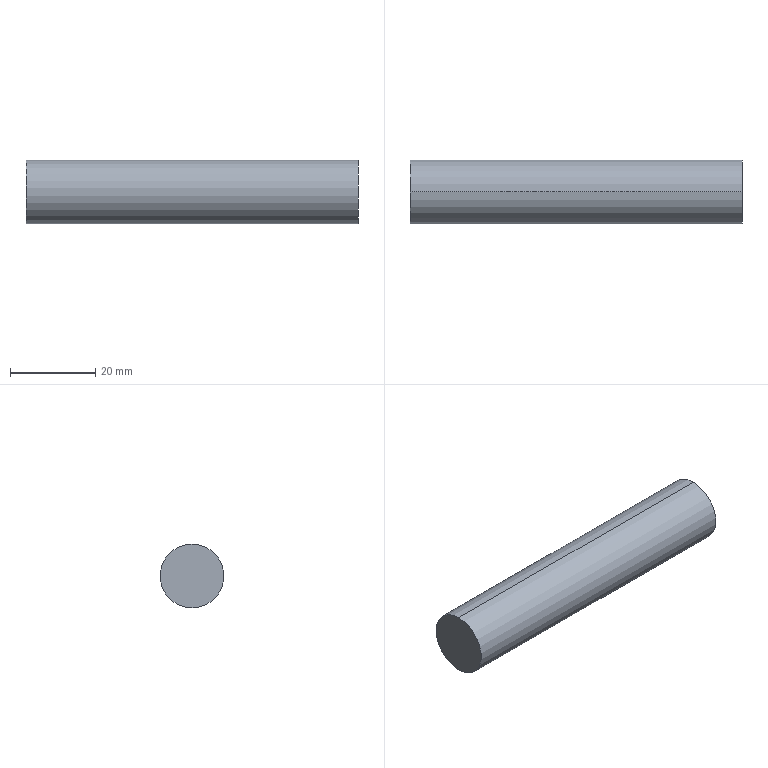Part | STEP file | PN_0018 (shaft rod) | 1 solid | 4 faces | box 78 x 15 x 15 mm | volume 13784 mm3 | cylinder 2 | plane 2 | commonest cylinder face diameters 15 x2
STEP:
#1=CARTESIAN_POINT('',(0.,0.,0.));
#2=DIRECTION('',(0.,0.,1.));
#3=DIRECTION('',(1.,0.,0.));
#4=AXIS2_PLACEMENT_3D('',#1,#2,#3);
#5=CARTESIAN_POINT('',(39.,0.,-7.5));
#6=VERTEX_POINT('',#5);
#7=CARTESIAN_POINT('',(39.,0.,7.5));
#8=VERTEX_POINT('',#7);
#9=CARTESIAN_POINT('',(39.,0.,0.));
#10=DIRECTION('',(1.,0.,0.));
#11=DIRECTION('',(0.,0.,-1.));
#12=AXIS2_PLACEMENT_3D('',#9,#10,#11);
#13=CIRCLE('',#12,7.5);
#14=CARTESIAN_POINT('',(39.,0.,0.));
#15=DIRECTION('',(-1.,0.,0.));
#16=DIRECTION('',(0.,0.,1.));
#17=AXIS2_PLACEMENT_3D('',#14,#15,#16);
#18=CYLINDRICAL_SURFACE('',#17,7.5);
#19=CARTESIAN_POINT('',(3.142,0.));
#20=DIRECTION('',(-1.,0.));
#21=VECTOR('',#20,1.);
#22=LINE('',#19,#21);
#23=(GEOMETRIC_REPRESENTATION_CONTEXT(2)PARAMETRIC_REPRESENTATION_CONTEXT()REPRESENTATION_CONTEXT('',''));
#24=DEFINITIONAL_REPRESENTATION('',(#22),#23);
#25=PCURVE('',#18,#24);
#26=CARTESIAN_POINT('',(39.,0.,0.));
#27=DIRECTION('',(1.,0.,0.));
#28=DIRECTION('',(0.,0.,-1.));
#29=AXIS2_PLACEMENT_3D('',#26,#27,#28);
#30=PLANE('',#29);
#31=CARTESIAN_POINT('',(0.,0.));
#32=DIRECTION('',(1.,0.));
#33=AXIS2_PLACEMENT_2D('',#31,#32);
#34=CIRCLE('',#33,7.5);
#35=(GEOMETRIC_REPRESENTATION_CONTEXT(2)PARAMETRIC_REPRESENTATION_CONTEXT()REPRESENTATION_CONTEXT('',''));
#36=DEFINITIONAL_REPRESENTATION('',(#34),#35);
#37=PCURVE('',#30,#36);
#38=SURFACE_CURVE('',#13,(#25,#37),.PCURVE_S1.);
#39=EDGE_CURVE('',#6,#8,#38,.T.);
#40=ORIENTED_EDGE('',*,*,#39,.F.);
#41=CARTESIAN_POINT('',(-39.,0.,-7.5));
#42=VERTEX_POINT('',#41);
#43=CARTESIAN_POINT('',(39.,0.,-7.5));
#44=DIRECTION('',(-1.,0.,0.));
#45=VECTOR('',#44,1.);
#46=LINE('',#43,#45);
#47=CARTESIAN_POINT('',(3.142,0.));
#48=DIRECTION('',(0.,1.));
#49=VECTOR('',#48,1.);
#50=LINE('',#47,#49);
#51=(GEOMETRIC_REPRESENTATION_CONTEXT(2)PARAMETRIC_REPRESENTATION_CONTEXT()REPRESENTATION_CONTEXT('',''));
#52=DEFINITIONAL_REPRESENTATION('',(#50),#51);
#53=PCURVE('',#18,#52);
#54=CARTESIAN_POINT('',(39.,0.,0.));
#55=DIRECTION('',(-1.,0.,0.));
#56=DIRECTION('',(0.,0.,1.));
#57=AXIS2_PLACEMENT_3D('',#54,#55,#56);
#58=CYLINDRICAL_SURFACE('',#57,7.5);
#59=CARTESIAN_POINT('',(3.142,0.));
#60=DIRECTION('',(0.,1.));
#61=VECTOR('',#60,1.);
#62=LINE('',#59,#61);
#63=(GEOMETRIC_REPRESENTATION_CONTEXT(2)PARAMETRIC_REPRESENTATION_CONTEXT()REPRESENTATION_CONTEXT('',''));
#64=DEFINITIONAL_REPRESENTATION('',(#62),#63);
#65=PCURVE('',#58,#64);
#66=SURFACE_CURVE('',#46,(#53,#65),.PCURVE_S1.);
#67=EDGE_CURVE('',#6,#42,#66,.T.);
#68=ORIENTED_EDGE('',*,*,#67,.T.);
#69=CARTESIAN_POINT('',(-39.,0.,7.5));
#70=VERTEX_POINT('',#69);
#71=CARTESIAN_POINT('',(-39.,0.,0.));
#72=DIRECTION('',(1.,0.,0.));
#73=DIRECTION('',(0.,0.,-1.));
#74=AXIS2_PLACEMENT_3D('',#71,#72,#73);
#75=CIRCLE('',#74,7.5);
#76=CARTESIAN_POINT('',(3.142,78.));
#77=DIRECTION('',(-1.,0.));
#78=VECTOR('',#77,1.);
#79=LINE('',#76,#78);
#80=(GEOMETRIC_REPRESENTATION_CONTEXT(2)PARAMETRIC_REPRESENTATION_CONTEXT()REPRESENTATION_CONTEXT('',''));
#81=DEFINITIONAL_REPRESENTATION('',(#79),#80);
#82=PCURVE('',#18,#81);
#83=CARTESIAN_POINT('',(-39.,0.,0.));
#84=DIRECTION('',(1.,0.,0.));
#85=DIRECTION('',(0.,0.,-1.));
#86=AXIS2_PLACEMENT_3D('',#83,#84,#85);
#87=PLANE('',#86);
#88=CARTESIAN_POINT('',(0.,0.));
#89=DIRECTION('',(1.,0.));
#90=AXIS2_PLACEMENT_2D('',#88,#89);
#91=CIRCLE('',#90,7.5);
#92=(GEOMETRIC_REPRESENTATION_CONTEXT(2)PARAMETRIC_REPRESENTATION_CONTEXT()REPRESENTATION_CONTEXT('',''));
#93=DEFINITIONAL_REPRESENTATION('',(#91),#92);
#94=PCURVE('',#87,#93);
#95=SURFACE_CURVE('',#75,(#82,#94),.PCURVE_S1.);
#96=EDGE_CURVE('',#42,#70,#95,.T.);
#97=ORIENTED_EDGE('',*,*,#96,.T.);
#98=CARTESIAN_POINT('',(39.,0.,7.5));
#99=DIRECTION('',(-1.,0.,0.));
#100=VECTOR('',#99,1.);
#101=LINE('',#98,#100);
#102=CARTESIAN_POINT('',(0.,0.));
#103=DIRECTION('',(0.,1.));
#104=VECTOR('',#103,1.);
#105=LINE('',#102,#104);
#106=(GEOMETRIC_REPRESENTATION_CONTEXT(2)PARAMETRIC_REPRESENTATION_CONTEXT()REPRESENTATION_CONTEXT('',''));
#107=DEFINITIONAL_REPRESENTATION('',(#105),#106);
#108=PCURVE('',#18,#107);
#109=CARTESIAN_POINT('',(6.283,0.));
#110=DIRECTION('',(0.,1.));
#111=VECTOR('',#110,1.);
#112=LINE('',#109,#111);
#113=(GEOMETRIC_REPRESENTATION_CONTEXT(2)PARAMETRIC_REPRESENTATION_CONTEXT()REPRESENTATION_CONTEXT('',''));
#114=DEFINITIONAL_REPRESENTATION('',(#112),#113);
#115=PCURVE('',#58,#114);
#116=SURFACE_CURVE('',#101,(#108,#115),.PCURVE_S1.);
#117=EDGE_CURVE('',#8,#70,#116,.T.);
#118=ORIENTED_EDGE('',*,*,#117,.F.);
#119=EDGE_LOOP('',(#40,#68,#97,#118));
#120=FACE_BOUND('',#119,.T.);
#121=ADVANCED_FACE('',(#120),#18,.T.);
#122=ORIENTED_EDGE('',*,*,#67,.F.);
#123=CARTESIAN_POINT('',(39.,0.,0.));
#124=DIRECTION('',(1.,0.,0.));
#125=DIRECTION('',(0.,0.,-1.));
#126=AXIS2_PLACEMENT_3D('',#123,#124,#125);
#127=CIRCLE('',#126,7.5);
#128=CARTESIAN_POINT('',(9.425,0.));
#129=DIRECTION('',(-1.,0.));
#130=VECTOR('',#129,1.);
#131=LINE('',#128,#130);
#132=(GEOMETRIC_REPRESENTATION_CONTEXT(2)PARAMETRIC_REPRESENTATION_CONTEXT()REPRESENTATION_CONTEXT('',''));
#133=DEFINITIONAL_REPRESENTATION('',(#131),#132);
#134=PCURVE('',#58,#133);
#135=CARTESIAN_POINT('',(0.,0.));
#136=DIRECTION('',(1.,0.));
#137=AXIS2_PLACEMENT_2D('',#135,#136);
#138=CIRCLE('',#137,7.5);
#139=(GEOMETRIC_REPRESENTATION_CONTEXT(2)PARAMETRIC_REPRESENTATION_CONTEXT()REPRESENTATION_CONTEXT('',''));
#140=DEFINITIONAL_REPRESENTATION('',(#138),#139);
#141=PCURVE('',#30,#140);
#142=SURFACE_CURVE('',#127,(#134,#141),.PCURVE_S1.);
#143=EDGE_CURVE('',#8,#6,#142,.T.);
#144=ORIENTED_EDGE('',*,*,#143,.F.);
#145=ORIENTED_EDGE('',*,*,#117,.T.);
#146=CARTESIAN_POINT('',(-39.,0.,0.));
#147=DIRECTION('',(1.,0.,0.));
#148=DIRECTION('',(0.,0.,-1.));
#149=AXIS2_PLACEMENT_3D('',#146,#147,#148);
#150=CIRCLE('',#149,7.5);
#151=CARTESIAN_POINT('',(9.425,78.));
#152=DIRECTION('',(-1.,0.));
#153=VECTOR('',#152,1.);
#154=LINE('',#151,#153);
#155=(GEOMETRIC_REPRESENTATION_CONTEXT(2)PARAMETRIC_REPRESENTATION_CONTEXT()REPRESENTATION_CONTEXT('',''));
#156=DEFINITIONAL_REPRESENTATION('',(#154),#155);
#157=PCURVE('',#58,#156);
#158=CARTESIAN_POINT('',(0.,0.));
#159=DIRECTION('',(1.,0.));
#160=AXIS2_PLACEMENT_2D('',#158,#159);
#161=CIRCLE('',#160,7.5);
#162=(GEOMETRIC_REPRESENTATION_CONTEXT(2)PARAMETRIC_REPRESENTATION_CONTEXT()REPRESENTATION_CONTEXT('',''));
#163=DEFINITIONAL_REPRESENTATION('',(#161),#162);
#164=PCURVE('',#87,#163);
#165=SURFACE_CURVE('',#150,(#157,#164),.PCURVE_S1.);
#166=EDGE_CURVE('',#70,#42,#165,.T.);
#167=ORIENTED_EDGE('',*,*,#166,.T.);
#168=EDGE_LOOP('',(#122,#144,#145,#167));
#169=FACE_BOUND('',#168,.T.);
#170=ADVANCED_FACE('',(#169),#58,.T.);
#171=ORIENTED_EDGE('',*,*,#143,.T.);
#172=ORIENTED_EDGE('',*,*,#39,.T.);
#173=EDGE_LOOP('',(#171,#172));
#174=FACE_BOUND('',#173,.T.);
#175=ADVANCED_FACE('',(#174),#30,.T.);
#176=ORIENTED_EDGE('',*,*,#166,.F.);
#177=ORIENTED_EDGE('',*,*,#96,.F.);
#178=EDGE_LOOP('',(#176,#177));
#179=FACE_BOUND('',#178,.T.);
#180=ADVANCED_FACE('',(#179),#87,.F.);
#181=CLOSED_SHELL('',(#121,#170,#175,#180));
#182=MANIFOLD_SOLID_BREP('',#181);
#183=(LENGTH_UNIT()NAMED_UNIT(*)SI_UNIT(.MILLI.,.METRE.));
#184=UNCERTAINTY_MEASURE_WITH_UNIT(LENGTH_MEASURE(0.0000001),#183,'','');
#185=(NAMED_UNIT(*)PLANE_ANGLE_UNIT()SI_UNIT($,.RADIAN.));
#186=(NAMED_UNIT(*)SI_UNIT($,.STERADIAN.)SOLID_ANGLE_UNIT());
#187=(GEOMETRIC_REPRESENTATION_CONTEXT(3)GLOBAL_UNCERTAINTY_ASSIGNED_CONTEXT((#184))GLOBAL_UNIT_ASSIGNED_CONTEXT((#183,#185,#186))REPRESENTATION_CONTEXT('',''));
#188=ADVANCED_BREP_SHAPE_REPRESENTATION('',(#4,#182),#187);